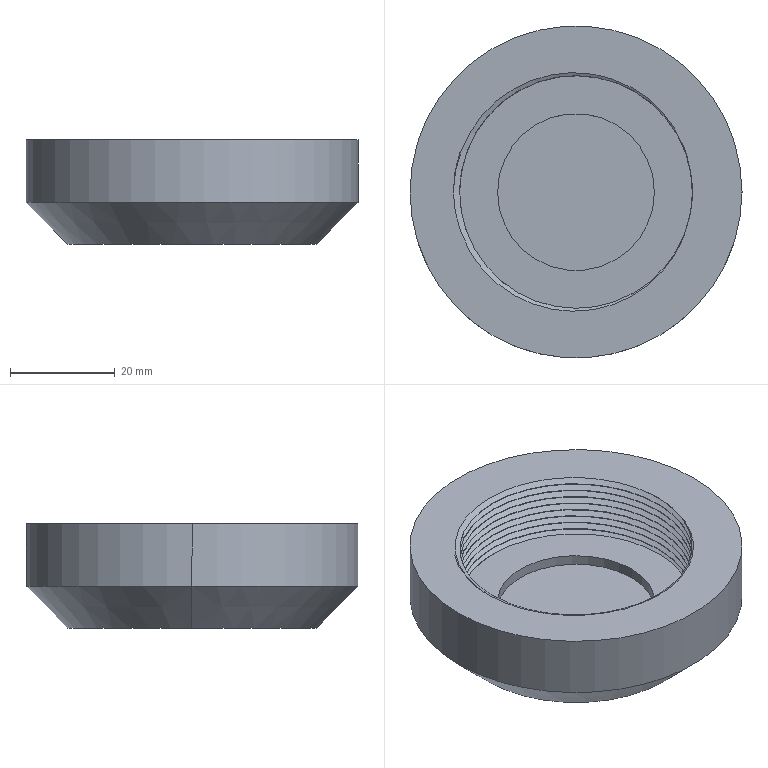Part | STEP file | output terminal cover plate^spray gun PTFE model | 1 solid | 33 faces | box 63.5 x 63.5 x 20 mm | volume 34764 mm3 | cylinder 23 | plane 5 | spline 3 | cone 2 | commonest cylinder face diameters 44.5 x19 30 x2 63.5 x2